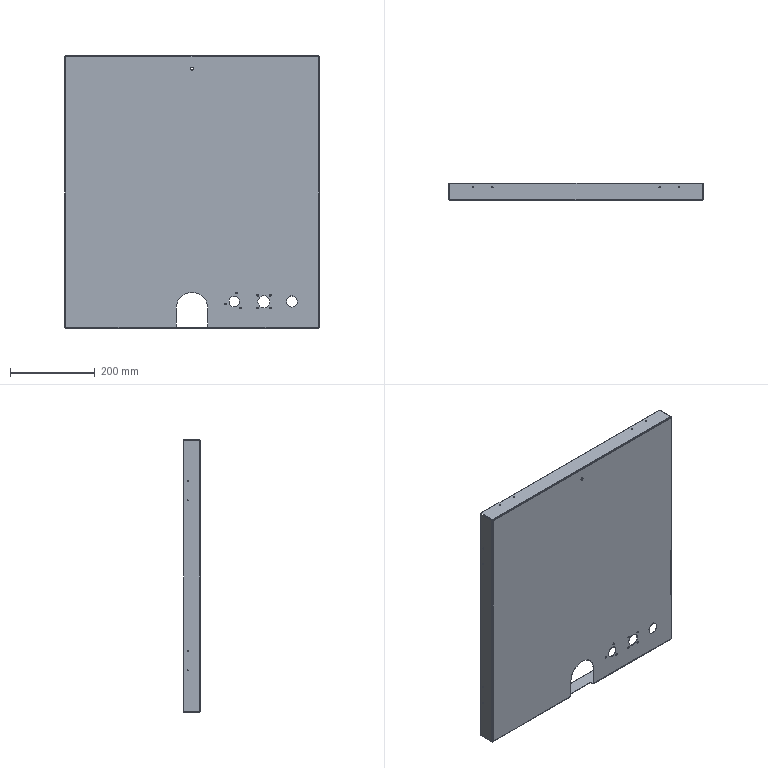Part | STEP file | JBJ-P-1011-05a | 1 solid | 74 faces | box 600 x 40 x 643 mm | volume 566077 mm3 | cylinder 38 | plane 28 | spline 8 | commonest cylinder face diameters 2.5 x8 3.2 x8 4 x7 2 x5 4.4 x5 6.5 x1